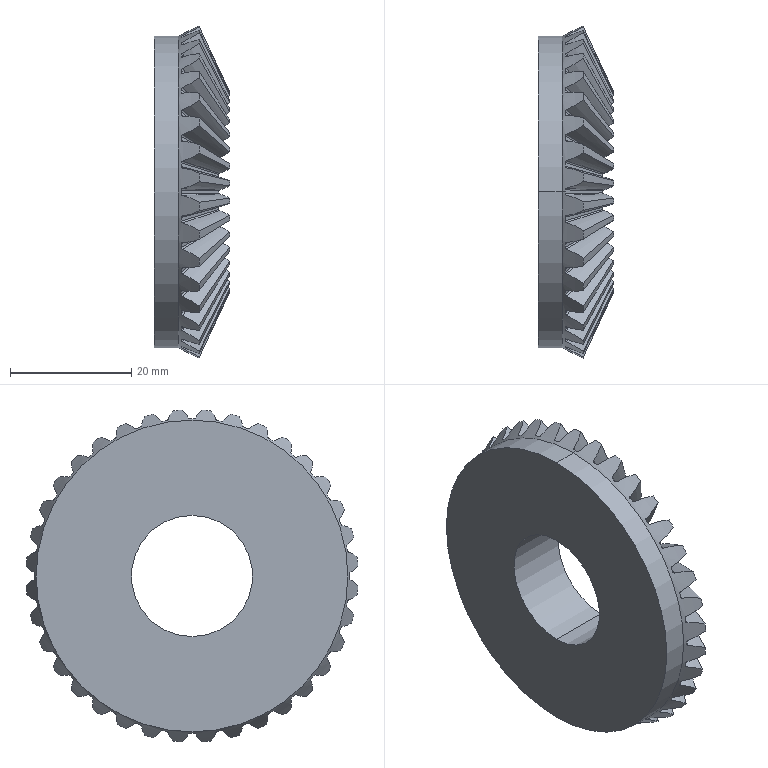Part | SolidWorks | features CirPattern 2, Cut 2, BlendCut 1, Boss 1, ICE 1, Revolution 1 | 1 solid | 226 faces | box 12.396 x 54.775 x 54.775 mm | volume 16791 mm3 | spline 180 | cone 40 | cylinder 4 | plane 2 | commonest cylinder face diameters 20 x2 51.428 x2